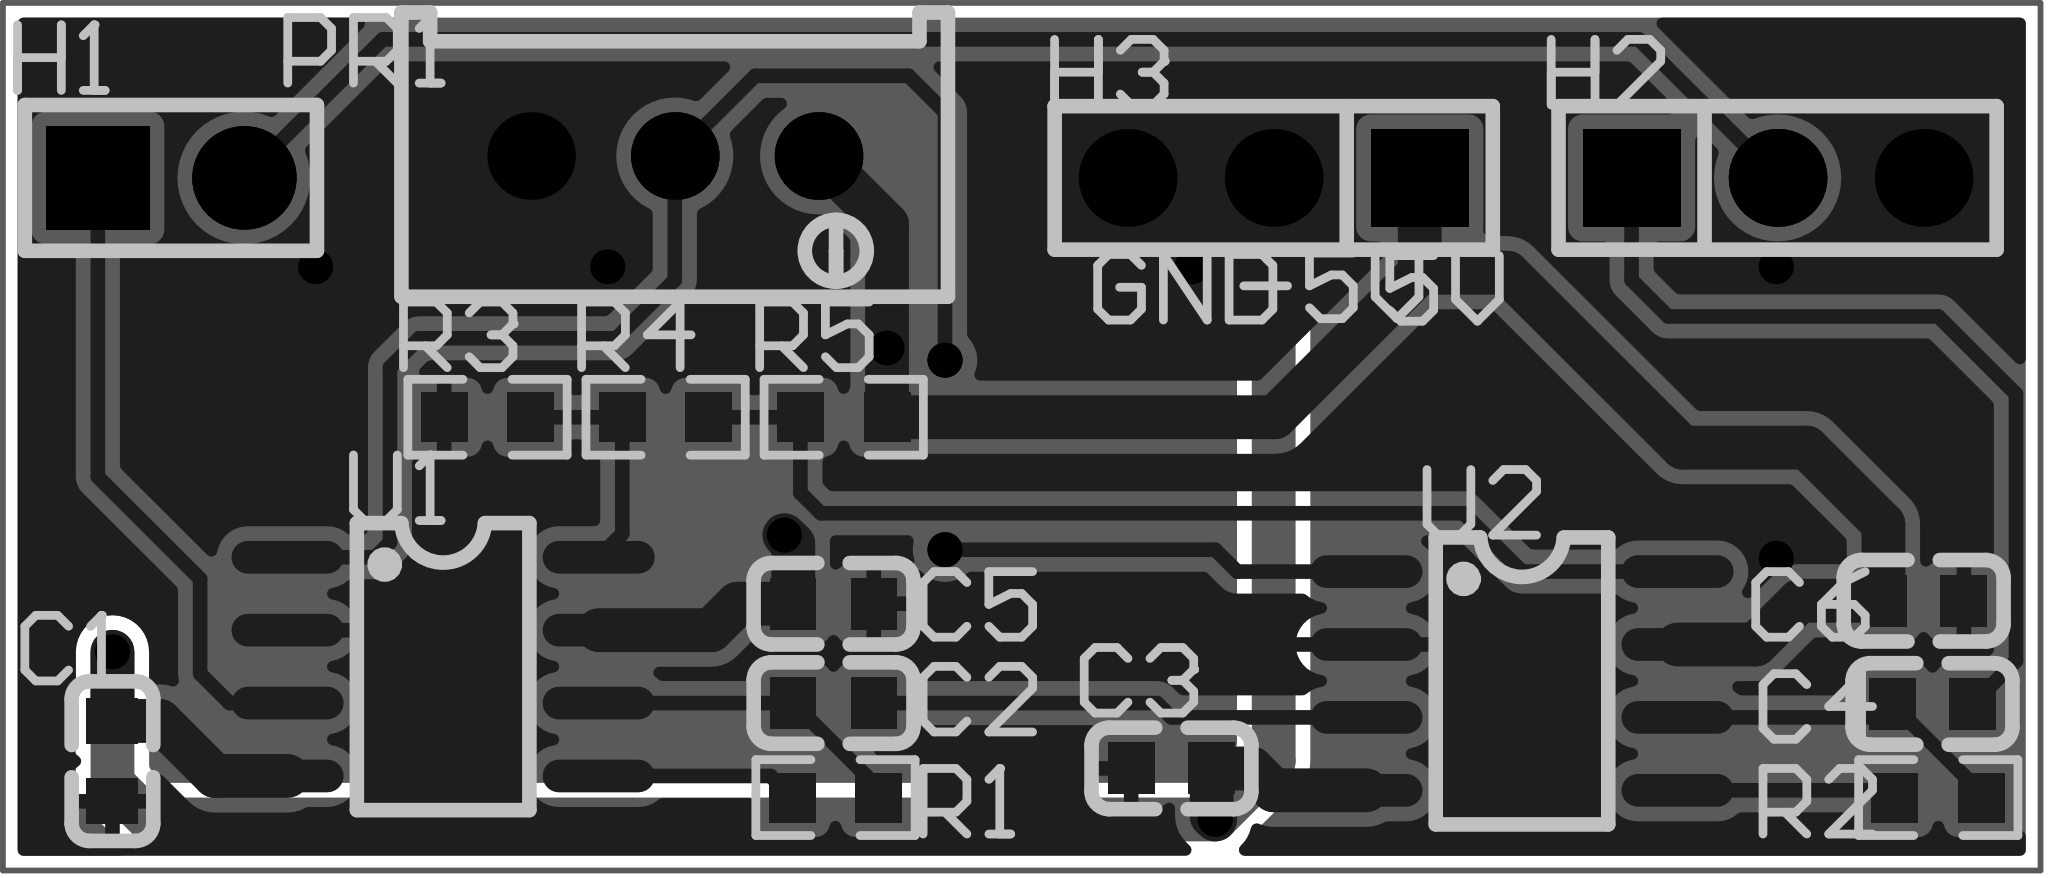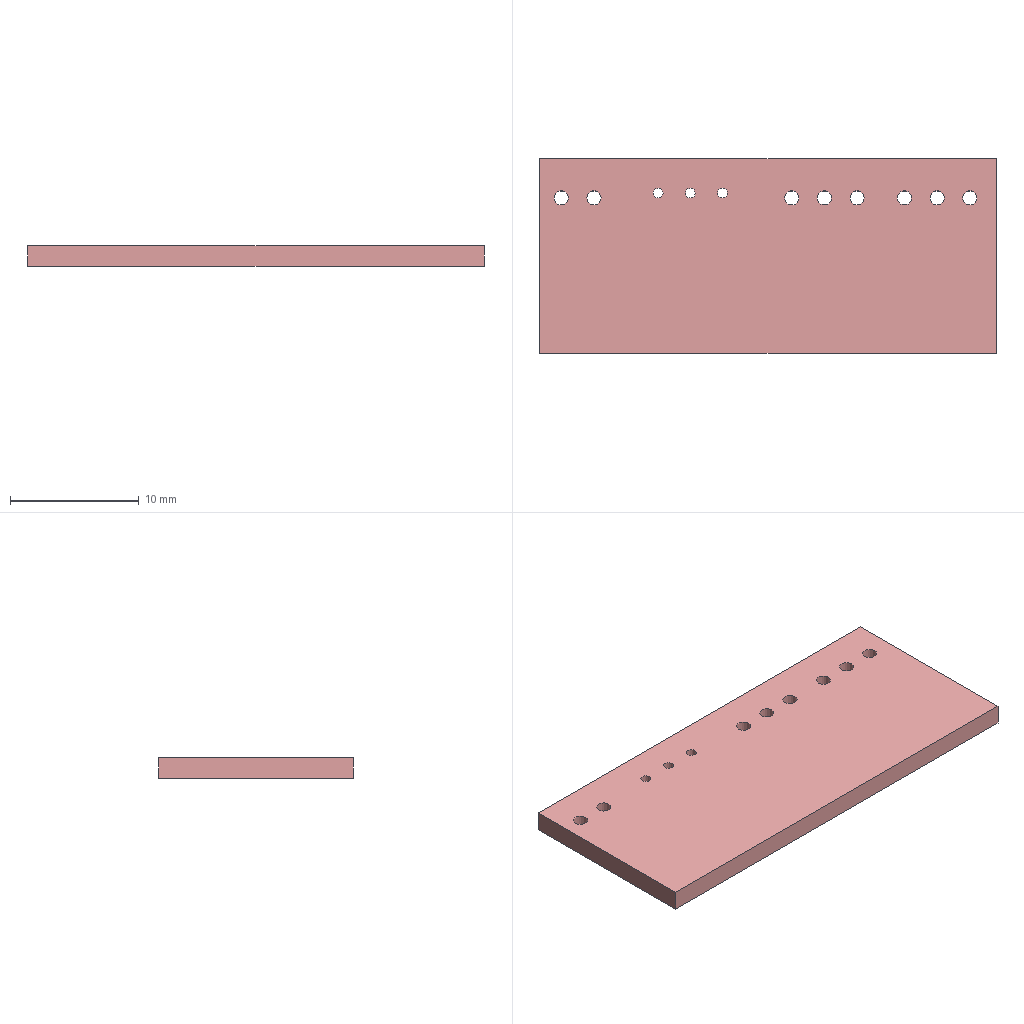Circuit board layout | Altium Designer | box 35.4 x 15.1 x 1.6 mm
Layer stack:
# Altium Designer layer stack of  (unit mm; dielectric type: 0 none, 1 core, 2 prepreg, 3 surface material)
index,name,kind,layer,copper_thickness_mm,dielectric_type,dielectric_thickness_mm,dielectric_material,dielectric_constant
0,Top Paste Mask Layer,other,,,,,,
1,Top Silkscreen Layer,other,,,,,,
2,Top Solder Mask Layer,dielectric,,,3,0.01,,3.3
3,Top Layer,copper,Top Layer,0.035,,,,
4,Dielectric1,dielectric,,,3,1.51,FR4,4.5
5,Bottom Layer,copper,Bottom Layer,0.035,,,,
6,Bottom Solder Mask Layer,dielectric,,,3,0.01,,3.3
7,Bottom Silkscreen Layer,other,,,,,,
8,Bottom Paste Mask Layer,other,,,,,,
# drill layer pairs: low layer,high layer
drill_pair,Top Layer,Bottom Layer
Part placement:
Designator,Comment,Layer,Footprint,Center-X(mm),Center-Y(mm),Rotation
C1,10uF,TopLayer,C0603,79.502,80.518,90
C2,10uF,TopLayer,C0603,92.042,81.529,0
C3,10uF,TopLayer,C0603,97.917,80.391,0
C4,10uF,TopLayer,C0603,111.152,81.514,0
C5,100nF,TopLayer,C0603,92.041,83.26,180
C6,100nF,TopLayer,C0603,110.998,83.312,180
H1,,TopLayer,HDR-TH_2P-P2.54-V-M-1,80.518,90.678,0
H2,,TopLayer,HDR-TH_3P-P2.54-V-M,108.458,90.678,0
H3,,TopLayer,HDR-TH_3P-P2.54-V-M,99.695,90.678,180
PR1,1kΩ,TopLayer,R_3296,89.281,91.059,180
R1,49.4K,TopLayer,R0603,92.075,79.883,0
R2,49.4K,TopLayer,R0603,111.252,79.883,0
R3,1K,TopLayer,R0603,86.024,86.509,0
R4,1K,TopLayer,R0603,89.121,86.509,0
R5,1K,TopLayer,R0603,92.218,86.509,0
U1,AD620N,TopLayer,SOIC-8_L5.0-W4.0-P1.27-LS6.0-BL,85.252,82.165,270
U2,AD620N,TopLayer,SOIC-8_L5.0-W4.0-P1.27-LS6.0-BL,104.013,81.915,270
Pad and via stacks:
# Altium Designer via and pad stacks of  (unit mm). Each distinct definition once, with the count of objects using it.
# via: kind,start_layer,end_layer,hole_mm,diameter_mm,mode(0 simple;1 top-mid-bottom;2 full stack),diameter_per_layer,count,example_net
# pad: kind,layer,hole_mm,hole_type(0 round;1 square;2 slot),plating,top_size,top_shape(1 round;2 rect;3 octagon;9 rounded rect),mid_size,bottom_size,mode,footprint,size_per_layer,count,example
pad,Top Layer,0,0,plated,0.8x0.9,2,0.8x0.9,0.8x0.9,0,C0603,,12,C1.2
pad,Top Layer,0,0,plated,0.8065x0.864,2,0.8065x0.864,0.8065x0.864,0,R0603,,10,R1.2
pad,Top Layer,0,0,plated,0.5684x1.95,1,0.5684x1.95,0.5684x1.95,0,SOIC-8_L5.0-W4.0-P1.27-LS6.0-BL,,16,U1.1
pad,Multi-Layer,1.1,0,plated,1.8x1.8,1,1.8x1.8,1.8x1.8,0,HDR-TH_2P-P2.54-V-M-1,,1,H1.2
pad,Multi-Layer,1.1,0,plated,1.8x1.8,2,1.8x1.8,1.8x1.8,0,HDR-TH_2P-P2.54-V-M-1,,1,H1.1
pad,Multi-Layer,1.1,0,plated,1.7x1.7,2,1.7x1.7,1.7x1.7,0,HDR-TH_3P-P2.54-V-M,,2,H2.1
pad,Multi-Layer,1.1,0,plated,1.7x1.7,1,1.7x1.7,1.7x1.7,0,HDR-TH_3P-P2.54-V-M,,4,H2.2
pad,Multi-Layer,0.762,0,plated,1.524x1.524,1,1.524x1.524,1.524x1.524,0,R_3296,,3,PR1.2
via,Top Layer,Bottom Layer,0.3048,0.61,0,,11,$1N16
Copper pours:
name,layer,net,type(0 solid;1 hatched;2 none)
Bottom Layer-GND,Bottom Layer,GND,0
Top Layer-GND,Top Layer,GND,0
Design rules, without the lines most boards share:
# Altium Designer design rules of  (exported by Altium Designer, unit mm)
# columns: name | kind | enabled | priority | scope1 | scope2 | descriptor | typed fields (field=value)
copperRegion | 20 | enabled | 1 | (InNet('GND')) | All | Polygon Connect Rule(Relief Connect )(Conductor Width=10mil) (Relief Angle=90 Angle) (Entries=4) (Air Gap Width=10mil) ((InNet('GND'))),(All) | connect_style(0=relief,1=direct,2=none)=0 relief_conductor_width=0.254 relief_entries=4